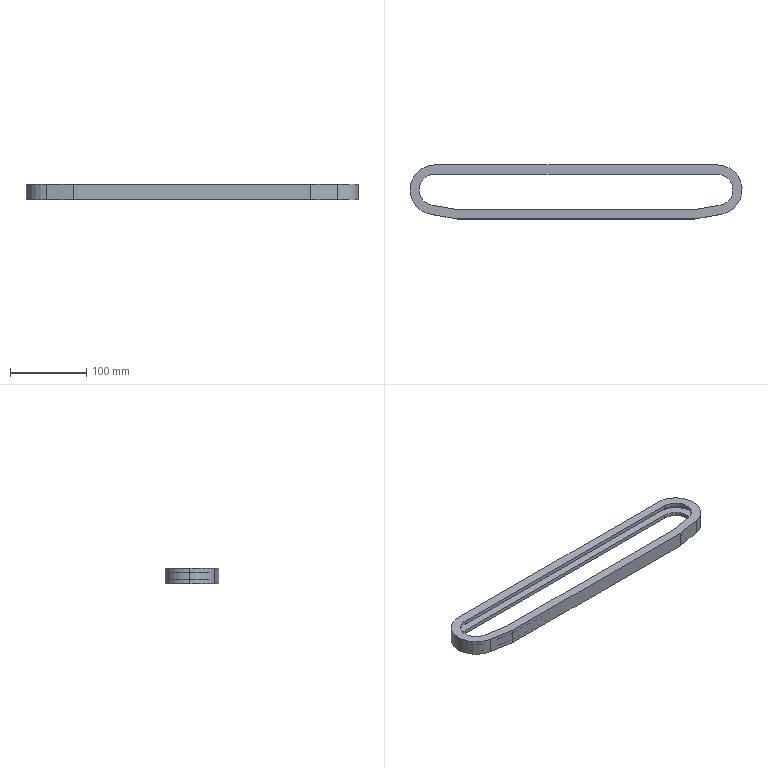Part | SolidWorks | features Extrusion 1, ICE 1 | 1 solid | 32 faces | box 435 x 70.699 x 20 mm | volume 118324 mm3 | plane 20 | cylinder 12 | commonest cylinder face diameters 41 x6 63 x3 65 x3
STEP:
#1=CARTESIAN_POINT('',(216.5,0.,-5.));
#2=VERTEX_POINT('',#1);
#3=CARTESIAN_POINT('',(185.,31.5,-5.));
#4=VERTEX_POINT('',#3);
#5=CARTESIAN_POINT('',(185.,0.,-5.));
#6=DIRECTION('',(0.,0.,1.));
#7=DIRECTION('',(1.,0.,0.));
#8=AXIS2_PLACEMENT_3D('',#5,#6,#7);
#9=CIRCLE('',#8,31.5);
#10=EDGE_CURVE('',#2,#4,#9,.T.);
#11=ORIENTED_EDGE('',*,*,#10,.F.);
#12=CARTESIAN_POINT('',(216.5,0.,5.));
#13=VERTEX_POINT('',#12);
#14=CARTESIAN_POINT('',(216.5,0.,-5.));
#15=DIRECTION('',(0.,0.,1.));
#16=VECTOR('',#15,1000.);
#17=LINE('',#14,#16);
#18=EDGE_CURVE('',#2,#13,#17,.T.);
#19=ORIENTED_EDGE('',*,*,#18,.T.);
#20=CARTESIAN_POINT('',(185.,31.5,5.));
#21=VERTEX_POINT('',#20);
#22=CARTESIAN_POINT('',(185.,0.,5.));
#23=DIRECTION('',(0.,0.,1.));
#24=DIRECTION('',(1.,0.,0.));
#25=AXIS2_PLACEMENT_3D('',#22,#23,#24);
#26=CIRCLE('',#25,31.5);
#27=EDGE_CURVE('',#13,#21,#26,.T.);
#28=ORIENTED_EDGE('',*,*,#27,.T.);
#29=CARTESIAN_POINT('',(185.,31.5,-5.));
#30=DIRECTION('',(0.,0.,1.));
#31=VECTOR('',#30,1000.);
#32=LINE('',#29,#31);
#33=EDGE_CURVE('',#4,#21,#32,.T.);
#34=ORIENTED_EDGE('',*,*,#33,.F.);
#35=EDGE_LOOP('',(#11,#19,#28,#34));
#36=FACE_OUTER_BOUND('',#35,.T.);
#37=CARTESIAN_POINT('',(185.,0.,-5.));
#38=DIRECTION('',(0.,0.,1.));
#39=DIRECTION('',(1.,0.,0.));
#40=AXIS2_PLACEMENT_3D('',#37,#38,#39);
#41=CYLINDRICAL_SURFACE('',#40,31.5);
#42=ADVANCED_FACE('',(#36),#41,.F.);
#43=CARTESIAN_POINT('',(-185.,20.5,10.));
#44=VERTEX_POINT('',#43);
#45=CARTESIAN_POINT('',(-205.5,0.,10.));
#46=VERTEX_POINT('',#45);
#47=CARTESIAN_POINT('',(-185.,0.,10.));
#48=DIRECTION('',(0.,0.,1.));
#49=DIRECTION('',(1.,0.,0.));
#50=AXIS2_PLACEMENT_3D('',#47,#48,#49);
#51=CIRCLE('',#50,20.5);
#52=EDGE_CURVE('',#44,#46,#51,.T.);
#53=ORIENTED_EDGE('',*,*,#52,.T.);
#54=CARTESIAN_POINT('',(-205.5,0.,5.));
#55=VERTEX_POINT('',#54);
#56=CARTESIAN_POINT('',(-205.5,0.,10.));
#57=DIRECTION('',(0.,0.,-1.));
#58=VECTOR('',#57,1000.);
#59=LINE('',#56,#58);
#60=EDGE_CURVE('',#46,#55,#59,.T.);
#61=ORIENTED_EDGE('',*,*,#60,.T.);
#62=CARTESIAN_POINT('',(-185.,20.5,5.));
#63=VERTEX_POINT('',#62);
#64=CARTESIAN_POINT('',(-185.,0.,5.));
#65=DIRECTION('',(0.,0.,1.));
#66=DIRECTION('',(1.,0.,0.));
#67=AXIS2_PLACEMENT_3D('',#64,#65,#66);
#68=CIRCLE('',#67,20.5);
#69=EDGE_CURVE('',#63,#55,#68,.T.);
#70=ORIENTED_EDGE('',*,*,#69,.F.);
#71=CARTESIAN_POINT('',(-185.,20.5,10.));
#72=DIRECTION('',(0.,0.,-1.));
#73=VECTOR('',#72,1000.);
#74=LINE('',#71,#73);
#75=EDGE_CURVE('',#44,#63,#74,.T.);
#76=ORIENTED_EDGE('',*,*,#75,.F.);
#77=EDGE_LOOP('',(#53,#61,#70,#76));
#78=FACE_OUTER_BOUND('',#77,.T.);
#79=CARTESIAN_POINT('',(-185.,0.,10.));
#80=DIRECTION('',(0.,0.,-1.));
#81=DIRECTION('',(-1.,0.,0.));
#82=AXIS2_PLACEMENT_3D('',#79,#80,#81);
#83=CYLINDRICAL_SURFACE('',#82,20.5);
#84=ADVANCED_FACE('',(#78),#83,.F.);
#85=CARTESIAN_POINT('',(-217.5,0.,10.));
#86=VERTEX_POINT('',#85);
#87=CARTESIAN_POINT('',(-190.644,-32.006,10.));
#88=VERTEX_POINT('',#87);
#89=CARTESIAN_POINT('',(-185.,0.,10.));
#90=DIRECTION('',(0.,0.,1.));
#91=DIRECTION('',(1.,0.,0.));
#92=AXIS2_PLACEMENT_3D('',#89,#90,#91);
#93=CIRCLE('',#92,32.5);
#94=EDGE_CURVE('',#86,#88,#93,.T.);
#95=ORIENTED_EDGE('',*,*,#94,.F.);
#96=CARTESIAN_POINT('',(-217.5,0.,-10.));
#97=VERTEX_POINT('',#96);
#98=CARTESIAN_POINT('',(-217.5,0.,10.));
#99=DIRECTION('',(0.,0.,-1.));
#100=VECTOR('',#99,1000.);
#101=LINE('',#98,#100);
#102=EDGE_CURVE('',#86,#97,#101,.T.);
#103=ORIENTED_EDGE('',*,*,#102,.T.);
#104=CARTESIAN_POINT('',(-190.644,-32.006,-10.));
#105=VERTEX_POINT('',#104);
#106=CARTESIAN_POINT('',(-185.,0.,-10.));
#107=DIRECTION('',(0.,0.,1.));
#108=DIRECTION('',(1.,0.,0.));
#109=AXIS2_PLACEMENT_3D('',#106,#107,#108);
#110=CIRCLE('',#109,32.5);
#111=EDGE_CURVE('',#97,#105,#110,.T.);
#112=ORIENTED_EDGE('',*,*,#111,.T.);
#113=CARTESIAN_POINT('',(-190.644,-32.006,10.));
#114=DIRECTION('',(0.,0.,-1.));
#115=VECTOR('',#114,1000.);
#116=LINE('',#113,#115);
#117=EDGE_CURVE('',#88,#105,#116,.T.);
#118=ORIENTED_EDGE('',*,*,#117,.F.);
#119=EDGE_LOOP('',(#95,#103,#112,#118));
#120=FACE_OUTER_BOUND('',#119,.T.);
#121=CARTESIAN_POINT('',(-185.,0.,10.));
#122=DIRECTION('',(0.,0.,-1.));
#123=DIRECTION('',(-1.,0.,0.));
#124=AXIS2_PLACEMENT_3D('',#121,#122,#123);
#125=CYLINDRICAL_SURFACE('',#124,32.5);
#126=ADVANCED_FACE('',(#120),#125,.T.);
#127=CARTESIAN_POINT('',(-185.,20.5,-5.));
#128=VERTEX_POINT('',#127);
#129=CARTESIAN_POINT('',(-205.5,0.,-5.));
#130=VERTEX_POINT('',#129);
#131=CARTESIAN_POINT('',(-185.,0.,-5.));
#132=DIRECTION('',(0.,0.,1.));
#133=DIRECTION('',(1.,0.,0.));
#134=AXIS2_PLACEMENT_3D('',#131,#132,#133);
#135=CIRCLE('',#134,20.5);
#136=EDGE_CURVE('',#128,#130,#135,.T.);
#137=ORIENTED_EDGE('',*,*,#136,.T.);
#138=CARTESIAN_POINT('',(-205.5,0.,-10.));
#139=VERTEX_POINT('',#138);
#140=CARTESIAN_POINT('',(-205.5,0.,10.));
#141=DIRECTION('',(0.,0.,-1.));
#142=VECTOR('',#141,1000.);
#143=LINE('',#140,#142);
#144=EDGE_CURVE('',#130,#139,#143,.T.);
#145=ORIENTED_EDGE('',*,*,#144,.T.);
#146=CARTESIAN_POINT('',(-185.,20.5,-10.));
#147=VERTEX_POINT('',#146);
#148=CARTESIAN_POINT('',(-185.,0.,-10.));
#149=DIRECTION('',(0.,0.,1.));
#150=DIRECTION('',(1.,0.,0.));
#151=AXIS2_PLACEMENT_3D('',#148,#149,#150);
#152=CIRCLE('',#151,20.5);
#153=EDGE_CURVE('',#147,#139,#152,.T.);
#154=ORIENTED_EDGE('',*,*,#153,.F.);
#155=CARTESIAN_POINT('',(-185.,20.5,10.));
#156=DIRECTION('',(0.,0.,-1.));
#157=VECTOR('',#156,1000.);
#158=LINE('',#155,#157);
#159=EDGE_CURVE('',#128,#147,#158,.T.);
#160=ORIENTED_EDGE('',*,*,#159,.F.);
#161=EDGE_LOOP('',(#137,#145,#154,#160));
#162=FACE_OUTER_BOUND('',#161,.T.);
#163=CARTESIAN_POINT('',(-185.,0.,10.));
#164=DIRECTION('',(0.,0.,-1.));
#165=DIRECTION('',(-1.,0.,0.));
#166=AXIS2_PLACEMENT_3D('',#163,#164,#165);
#167=CYLINDRICAL_SURFACE('',#166,20.5);
#168=ADVANCED_FACE('',(#162),#167,.F.);
#169=ORIENTED_EDGE('',*,*,#144,.F.);
#170=CARTESIAN_POINT('',(-188.56,-20.189,-5.));
#171=VERTEX_POINT('',#170);
#172=CARTESIAN_POINT('',(-185.,0.,-5.));
#173=DIRECTION('',(0.,0.,1.));
#174=DIRECTION('',(1.,0.,0.));
#175=AXIS2_PLACEMENT_3D('',#172,#173,#174);
#176=CIRCLE('',#175,20.5);
#177=EDGE_CURVE('',#130,#171,#176,.T.);
#178=ORIENTED_EDGE('',*,*,#177,.T.);
#179=CARTESIAN_POINT('',(-188.56,-20.189,-10.));
#180=VERTEX_POINT('',#179);
#181=CARTESIAN_POINT('',(-188.56,-20.189,10.));
#182=DIRECTION('',(0.,0.,-1.));
#183=VECTOR('',#182,1000.);
#184=LINE('',#181,#183);
#185=EDGE_CURVE('',#171,#180,#184,.T.);
#186=ORIENTED_EDGE('',*,*,#185,.T.);
#187=CARTESIAN_POINT('',(-185.,0.,-10.));
#188=DIRECTION('',(0.,0.,1.));
#189=DIRECTION('',(1.,0.,0.));
#190=AXIS2_PLACEMENT_3D('',#187,#188,#189);
#191=CIRCLE('',#190,20.5);
#192=EDGE_CURVE('',#139,#180,#191,.T.);
#193=ORIENTED_EDGE('',*,*,#192,.F.);
#194=EDGE_LOOP('',(#169,#178,#186,#193));
#195=FACE_OUTER_BOUND('',#194,.T.);
#196=CARTESIAN_POINT('',(-185.,0.,10.));
#197=DIRECTION('',(0.,0.,-1.));
#198=DIRECTION('',(-1.,0.,0.));
#199=AXIS2_PLACEMENT_3D('',#196,#197,#198);
#200=CYLINDRICAL_SURFACE('',#199,20.5);
#201=ADVANCED_FACE('',(#195),#200,.F.);
#202=ORIENTED_EDGE('',*,*,#185,.F.);
#203=CARTESIAN_POINT('',(-154.475,-26.199,-5.));
#204=VERTEX_POINT('',#203);
#205=CARTESIAN_POINT('',(-154.475,-26.199,-5.));
#206=DIRECTION('',(0.9848,-0.1736,0.));
#207=VECTOR('',#206,1000.);
#208=LINE('',#205,#207);
#209=EDGE_CURVE('',#171,#204,#208,.T.);
#210=ORIENTED_EDGE('',*,*,#209,.T.);
#211=CARTESIAN_POINT('',(-154.475,-26.199,-10.));
#212=VERTEX_POINT('',#211);
#213=CARTESIAN_POINT('',(-154.475,-26.199,10.));
#214=DIRECTION('',(0.,0.,-1.));
#215=VECTOR('',#214,1000.);
#216=LINE('',#213,#215);
#217=EDGE_CURVE('',#204,#212,#216,.T.);
#218=ORIENTED_EDGE('',*,*,#217,.T.);
#219=CARTESIAN_POINT('',(-154.475,-26.199,-10.));
#220=DIRECTION('',(0.9848,-0.1736,0.));
#221=VECTOR('',#220,1000.);
#222=LINE('',#219,#221);
#223=EDGE_CURVE('',#180,#212,#222,.T.);
#224=ORIENTED_EDGE('',*,*,#223,.F.);
#225=EDGE_LOOP('',(#202,#210,#218,#224));
#226=FACE_OUTER_BOUND('',#225,.T.);
#227=CARTESIAN_POINT('',(-154.475,-26.199,10.));
#228=DIRECTION('',(0.1736,0.9848,0.));
#229=DIRECTION('',(-0.9848,0.1736,0.));
#230=AXIS2_PLACEMENT_3D('',#227,#228,#229);
#231=PLANE('',#230);
#232=ADVANCED_FACE('',(#226),#231,.T.);
#233=ORIENTED_EDGE('',*,*,#217,.F.);
#234=CARTESIAN_POINT('',(154.475,-26.199,-5.));
#235=VERTEX_POINT('',#234);
#236=CARTESIAN_POINT('',(-154.475,-26.199,-5.));
#237=DIRECTION('',(1.,0.,0.));
#238=VECTOR('',#237,1000.);
#239=LINE('',#236,#238);
#240=EDGE_CURVE('',#204,#235,#239,.T.);
#241=ORIENTED_EDGE('',*,*,#240,.T.);
#242=CARTESIAN_POINT('',(154.475,-26.199,-10.));
#243=VERTEX_POINT('',#242);
#244=CARTESIAN_POINT('',(154.475,-26.199,10.));
#245=DIRECTION('',(0.,0.,-1.));
#246=VECTOR('',#245,1000.);
#247=LINE('',#244,#246);
#248=EDGE_CURVE('',#235,#243,#247,.T.);
#249=ORIENTED_EDGE('',*,*,#248,.T.);
#250=CARTESIAN_POINT('',(-154.475,-26.199,-10.));
#251=DIRECTION('',(1.,0.,0.));
#252=VECTOR('',#251,1000.);
#253=LINE('',#250,#252);
#254=EDGE_CURVE('',#212,#243,#253,.T.);
#255=ORIENTED_EDGE('',*,*,#254,.F.);
#256=EDGE_LOOP('',(#233,#241,#249,#255));
#257=FACE_OUTER_BOUND('',#256,.T.);
#258=CARTESIAN_POINT('',(-154.475,-26.199,10.));
#259=DIRECTION('',(0.,1.,0.));
#260=DIRECTION('',(0.,0.,1.));
#261=AXIS2_PLACEMENT_3D('',#258,#259,#260);
#262=PLANE('',#261);
#263=ADVANCED_FACE('',(#257),#262,.T.);
#264=ORIENTED_EDGE('',*,*,#248,.F.);
#265=CARTESIAN_POINT('',(188.56,-20.189,-5.));
#266=VERTEX_POINT('',#265);
#267=CARTESIAN_POINT('',(154.475,-26.199,-5.));
#268=DIRECTION('',(0.9848,0.1736,0.));
#269=VECTOR('',#268,1000.);
#270=LINE('',#267,#269);
#271=EDGE_CURVE('',#235,#266,#270,.T.);
#272=ORIENTED_EDGE('',*,*,#271,.T.);
#273=CARTESIAN_POINT('',(188.56,-20.189,-10.));
#274=VERTEX_POINT('',#273);
#275=CARTESIAN_POINT('',(188.56,-20.189,10.));
#276=DIRECTION('',(0.,0.,-1.));
#277=VECTOR('',#276,1000.);
#278=LINE('',#275,#277);
#279=EDGE_CURVE('',#266,#274,#278,.T.);
#280=ORIENTED_EDGE('',*,*,#279,.T.);
#281=CARTESIAN_POINT('',(154.475,-26.199,-10.));
#282=DIRECTION('',(0.9848,0.1736,0.));
#283=VECTOR('',#282,1000.);
#284=LINE('',#281,#283);
#285=EDGE_CURVE('',#243,#274,#284,.T.);
#286=ORIENTED_EDGE('',*,*,#285,.F.);
#287=EDGE_LOOP('',(#264,#272,#280,#286));
#288=FACE_OUTER_BOUND('',#287,.T.);
#289=CARTESIAN_POINT('',(154.475,-26.199,10.));
#290=DIRECTION('',(-0.1736,0.9848,0.));
#291=DIRECTION('',(-0.9848,-0.1736,0.));
#292=AXIS2_PLACEMENT_3D('',#289,#290,#291);
#293=PLANE('',#292);
#294=ADVANCED_FACE('',(#288),#293,.T.);
#295=ORIENTED_EDGE('',*,*,#279,.F.);
#296=CARTESIAN_POINT('',(185.,20.5,-5.));
#297=VERTEX_POINT('',#296);
#298=CARTESIAN_POINT('',(185.,0.,-5.));
#299=DIRECTION('',(0.,0.,1.));
#300=DIRECTION('',(1.,0.,0.));
#301=AXIS2_PLACEMENT_3D('',#298,#299,#300);
#302=CIRCLE('',#301,20.5);
#303=EDGE_CURVE('',#266,#297,#302,.T.);
#304=ORIENTED_EDGE('',*,*,#303,.T.);
#305=CARTESIAN_POINT('',(185.,20.5,-10.));
#306=VERTEX_POINT('',#305);
#307=CARTESIAN_POINT('',(185.,20.5,10.));
#308=DIRECTION('',(0.,0.,-1.));
#309=VECTOR('',#308,1000.);
#310=LINE('',#307,#309);
#311=EDGE_CURVE('',#297,#306,#310,.T.);
#312=ORIENTED_EDGE('',*,*,#311,.T.);
#313=CARTESIAN_POINT('',(185.,0.,-10.));
#314=DIRECTION('',(0.,0.,1.));
#315=DIRECTION('',(-1.,0.,0.));
#316=AXIS2_PLACEMENT_3D('',#313,#314,#315);
#317=CIRCLE('',#316,20.5);
#318=EDGE_CURVE('',#274,#306,#317,.T.);
#319=ORIENTED_EDGE('',*,*,#318,.F.);
#320=EDGE_LOOP('',(#295,#304,#312,#319));
#321=FACE_OUTER_BOUND('',#320,.T.);
#322=CARTESIAN_POINT('',(185.,0.,10.));
#323=DIRECTION('',(0.,0.,-1.));
#324=DIRECTION('',(-1.,0.,0.));
#325=AXIS2_PLACEMENT_3D('',#322,#323,#324);
#326=CYLINDRICAL_SURFACE('',#325,20.5);
#327=ADVANCED_FACE('',(#321),#326,.F.);
#328=ORIENTED_EDGE('',*,*,#311,.F.);
#329=CARTESIAN_POINT('',(-185.,20.5,-5.));
#330=DIRECTION('',(-1.,0.,0.));
#331=VECTOR('',#330,1000.);
#332=LINE('',#329,#331);
#333=EDGE_CURVE('',#297,#128,#332,.T.);
#334=ORIENTED_EDGE('',*,*,#333,.T.);
#335=ORIENTED_EDGE('',*,*,#159,.T.);
#336=CARTESIAN_POINT('',(-185.,20.5,-10.));
#337=DIRECTION('',(-1.,0.,0.));
#338=VECTOR('',#337,1000.);
#339=LINE('',#336,#338);
#340=EDGE_CURVE('',#306,#147,#339,.T.);
#341=ORIENTED_EDGE('',*,*,#340,.F.);
#342=EDGE_LOOP('',(#328,#334,#335,#341));
#343=FACE_OUTER_BOUND('',#342,.T.);
#344=CARTESIAN_POINT('',(-185.,20.5,10.));
#345=DIRECTION('',(0.,-1.,0.));
#346=DIRECTION('',(0.,0.,-1.));
#347=AXIS2_PLACEMENT_3D('',#344,#345,#346);
#348=PLANE('',#347);
#349=ADVANCED_FACE('',(#343),#348,.T.);
#350=CARTESIAN_POINT('',(-185.,32.5,10.));
#351=VERTEX_POINT('',#350);
#352=CARTESIAN_POINT('',(-185.,0.,10.));
#353=DIRECTION('',(0.,0.,1.));
#354=DIRECTION('',(1.,0.,0.));
#355=AXIS2_PLACEMENT_3D('',#352,#353,#354);
#356=CIRCLE('',#355,32.5);
#357=EDGE_CURVE('',#351,#86,#356,.T.);
#358=ORIENTED_EDGE('',*,*,#357,.T.);
#359=ORIENTED_EDGE('',*,*,#94,.T.);
#360=CARTESIAN_POINT('',(-155.525,-38.199,10.));
#361=VERTEX_POINT('',#360);
#362=CARTESIAN_POINT('',(-155.525,-38.199,10.));
#363=DIRECTION('',(0.9848,-0.1736,0.));
#364=VECTOR('',#363,1000.);
#365=LINE('',#362,#364);
#366=EDGE_CURVE('',#88,#361,#365,.T.);
#367=ORIENTED_EDGE('',*,*,#366,.T.);
#368=CARTESIAN_POINT('',(155.525,-38.199,10.));
#369=VERTEX_POINT('',#368);
#370=CARTESIAN_POINT('',(-155.525,-38.199,10.));
#371=DIRECTION('',(1.,0.,0.));
#372=VECTOR('',#371,1000.);
#373=LINE('',#370,#372);
#374=EDGE_CURVE('',#361,#369,#373,.T.);
#375=ORIENTED_EDGE('',*,*,#374,.T.);
#376=CARTESIAN_POINT('',(190.644,-32.006,10.));
#377=VERTEX_POINT('',#376);
#378=CARTESIAN_POINT('',(155.525,-38.199,10.));
#379=DIRECTION('',(0.9848,0.1736,0.));
#380=VECTOR('',#379,1000.);
#381=LINE('',#378,#380);
#382=EDGE_CURVE('',#369,#377,#381,.T.);
#383=ORIENTED_EDGE('',*,*,#382,.T.);
#384=CARTESIAN_POINT('',(185.,32.5,10.));
#385=VERTEX_POINT('',#384);
#386=CARTESIAN_POINT('',(185.,0.,10.));
#387=DIRECTION('',(0.,0.,1.));
#388=DIRECTION('',(-1.,0.,0.));
#389=AXIS2_PLACEMENT_3D('',#386,#387,#388);
#390=CIRCLE('',#389,32.5);
#391=EDGE_CURVE('',#377,#385,#390,.T.);
#392=ORIENTED_EDGE('',*,*,#391,.T.);
#393=CARTESIAN_POINT('',(-185.,32.5,10.));
#394=DIRECTION('',(-1.,0.,0.));
#395=VECTOR('',#394,1000.);
#396=LINE('',#393,#395);
#397=EDGE_CURVE('',#385,#351,#396,.T.);
#398=ORIENTED_EDGE('',*,*,#397,.T.);
#399=EDGE_LOOP('',(#358,#359,#367,#375,#383,#392,#398));
#400=FACE_OUTER_BOUND('',#399,.T.);
#401=CARTESIAN_POINT('',(-188.56,-20.189,10.));
#402=VERTEX_POINT('',#401);
#403=CARTESIAN_POINT('',(-154.475,-26.199,10.));
#404=VERTEX_POINT('',#403);
#405=CARTESIAN_POINT('',(-154.475,-26.199,10.));
#406=DIRECTION('',(0.9848,-0.1736,0.));
#407=VECTOR('',#406,1000.);
#408=LINE('',#405,#407);
#409=EDGE_CURVE('',#402,#404,#408,.T.);
#410=ORIENTED_EDGE('',*,*,#409,.F.);
#411=CARTESIAN_POINT('',(-185.,0.,10.));
#412=DIRECTION('',(0.,0.,1.));
#413=DIRECTION('',(1.,0.,0.));
#414=AXIS2_PLACEMENT_3D('',#411,#412,#413);
#415=CIRCLE('',#414,20.5);
#416=EDGE_CURVE('',#46,#402,#415,.T.);
#417=ORIENTED_EDGE('',*,*,#416,.F.);
#418=ORIENTED_EDGE('',*,*,#52,.F.);
#419=CARTESIAN_POINT('',(185.,20.5,10.));
#420=VERTEX_POINT('',#419);
#421=CARTESIAN_POINT('',(-185.,20.5,10.));
#422=DIRECTION('',(-1.,0.,0.));
#423=VECTOR('',#422,1000.);
#424=LINE('',#421,#423);
#425=EDGE_CURVE('',#420,#44,#424,.T.);
#426=ORIENTED_EDGE('',*,*,#425,.F.);
#427=CARTESIAN_POINT('',(188.56,-20.189,10.));
#428=VERTEX_POINT('',#427);
#429=CARTESIAN_POINT('',(185.,0.,10.));
#430=DIRECTION('',(0.,0.,1.));
#431=DIRECTION('',(-1.,0.,0.));
#432=AXIS2_PLACEMENT_3D('',#429,#430,#431);
#433=CIRCLE('',#432,20.5);
#434=EDGE_CURVE('',#428,#420,#433,.T.);
#435=ORIENTED_EDGE('',*,*,#434,.F.);
#436=CARTESIAN_POINT('',(154.475,-26.199,10.));
#437=VERTEX_POINT('',#436);
#438=CARTESIAN_POINT('',(154.475,-26.199,10.));
#439=DIRECTION('',(0.9848,0.1736,0.));
#440=VECTOR('',#439,1000.);
#441=LINE('',#438,#440);
#442=EDGE_CURVE('',#437,#428,#441,.T.);
#443=ORIENTED_EDGE('',*,*,#442,.F.);
#444=CARTESIAN_POINT('',(-154.475,-26.199,10.));
#445=DIRECTION('',(1.,0.,0.));
#446=VECTOR('',#445,1000.);
#447=LINE('',#444,#446);
#448=EDGE_CURVE('',#404,#437,#447,.T.);
#449=ORIENTED_EDGE('',*,*,#448,.F.);
#450=EDGE_LOOP('',(#410,#417,#418,#426,#435,#443,#449));
#451=FACE_BOUND('',#450,.T.);
#452=CARTESIAN_POINT('',(-185.,0.,10.));
#453=DIRECTION('',(0.,0.,1.));
#454=DIRECTION('',(1.,0.,0.));
#455=AXIS2_PLACEMENT_3D('',#452,#453,#454);
#456=PLANE('',#455);
#457=ADVANCED_FACE('',(#400,#451),#456,.T.);
#458=CARTESIAN_POINT('',(-185.,32.5,-10.));
#459=VERTEX_POINT('',#458);
#460=CARTESIAN_POINT('',(-185.,0.,-10.));
#461=DIRECTION('',(0.,0.,1.));
#462=DIRECTION('',(1.,0.,0.));
#463=AXIS2_PLACEMENT_3D('',#460,#461,#462);
#464=CIRCLE('',#463,32.5);
#465=EDGE_CURVE('',#459,#97,#464,.T.);
#466=ORIENTED_EDGE('',*,*,#465,.F.);
#467=CARTESIAN_POINT('',(185.,32.5,-10.));
#468=VERTEX_POINT('',#467);
#469=CARTESIAN_POINT('',(-185.,32.5,-10.));
#470=DIRECTION('',(-1.,0.,0.));
#471=VECTOR('',#470,1000.);
#472=LINE('',#469,#471);
#473=EDGE_CURVE('',#468,#459,#472,.T.);
#474=ORIENTED_EDGE('',*,*,#473,.F.);
#475=CARTESIAN_POINT('',(190.644,-32.006,-10.));
#476=VERTEX_POINT('',#475);
#477=CARTESIAN_POINT('',(185.,0.,-10.));
#478=DIRECTION('',(0.,0.,1.));
#479=DIRECTION('',(-1.,0.,0.));
#480=AXIS2_PLACEMENT_3D('',#477,#478,#479);
#481=CIRCLE('',#480,32.5);
#482=EDGE_CURVE('',#476,#468,#481,.T.);
#483=ORIENTED_EDGE('',*,*,#482,.F.);
#484=CARTESIAN_POINT('',(155.525,-38.199,-10.));
#485=VERTEX_POINT('',#484);
#486=CARTESIAN_POINT('',(155.525,-38.199,-10.));
#487=DIRECTION('',(0.9848,0.1736,0.));
#488=VECTOR('',#487,1000.);
#489=LINE('',#486,#488);
#490=EDGE_CURVE('',#485,#476,#489,.T.);
#491=ORIENTED_EDGE('',*,*,#490,.F.);
#492=CARTESIAN_POINT('',(-155.525,-38.199,-10.));
#493=VERTEX_POINT('',#492);
#494=CARTESIAN_POINT('',(-155.525,-38.199,-10.));
#495=DIRECTION('',(1.,0.,0.));
#496=VECTOR('',#495,1000.);
#497=LINE('',#494,#496);
#498=EDGE_CURVE('',#493,#485,#497,.T.);
#499=ORIENTED_EDGE('',*,*,#498,.F.);
#500=CARTESIAN_POINT('',(-155.525,-38.199,-10.));
#501=DIRECTION('',(0.9848,-0.1736,0.));
#502=VECTOR('',#501,1000.);
#503=LINE('',#500,#502);
#504=EDGE_CURVE('',#105,#493,#503,.T.);
#505=ORIENTED_EDGE('',*,*,#504,.F.);
#506=ORIENTED_EDGE('',*,*,#111,.F.);
#507=EDGE_LOOP('',(#466,#474,#483,#491,#499,#505,#506));
#508=FACE_OUTER_BOUND('',#507,.T.);
#509=ORIENTED_EDGE('',*,*,#153,.T.);
#510=ORIENTED_EDGE('',*,*,#192,.T.);
#511=ORIENTED_EDGE('',*,*,#223,.T.);
#512=ORIENTED_EDGE('',*,*,#254,.T.);
#513=ORIENTED_EDGE('',*,*,#285,.T.);
#514=ORIENTED_EDGE('',*,*,#318,.T.);
#515=ORIENTED_EDGE('',*,*,#340,.T.);
#516=EDGE_LOOP('',(#509,#510,#511,#512,#513,#514,#515));
#517=FACE_BOUND('',#516,.T.);
#518=CARTESIAN_POINT('',(-185.,0.,-10.));
#519=DIRECTION('',(0.,0.,1.));
#520=DIRECTION('',(1.,0.,0.));
#521=AXIS2_PLACEMENT_3D('',#518,#519,#520);
#522=PLANE('',#521);
#523=ADVANCED_FACE('',(#508,#517),#522,.F.);
#524=ORIENTED_EDGE('',*,*,#102,.F.);
#525=ORIENTED_EDGE('',*,*,#357,.F.);
#526=CARTESIAN_POINT('',(-185.,32.5,10.));
#527=DIRECTION('',(0.,0.,-1.));
#528=VECTOR('',#527,1000.);
#529=LINE('',#526,#528);
#530=EDGE_CURVE('',#351,#459,#529,.T.);
#531=ORIENTED_EDGE('',*,*,#530,.T.);
#532=ORIENTED_EDGE('',*,*,#465,.T.);
#533=EDGE_LOOP('',(#524,#525,#531,#532));
#534=FACE_OUTER_BOUND('',#533,.T.);
#535=CARTESIAN_POINT('',(-185.,0.,10.));
#536=DIRECTION('',(0.,0.,-1.));
#537=DIRECTION('',(-1.,0.,0.));
#538=AXIS2_PLACEMENT_3D('',#535,#536,#537);
#539=CYLINDRICAL_SURFACE('',#538,32.5);
#540=ADVANCED_FACE('',(#534),#539,.T.);
#541=ORIENTED_EDGE('',*,*,#504,.T.);
#542=CARTESIAN_POINT('',(-155.525,-38.199,10.));
#543=DIRECTION('',(0.,0.,-1.));
#544=VECTOR('',#543,1000.);
#545=LINE('',#542,#544);
#546=EDGE_CURVE('',#361,#493,#545,.T.);
#547=ORIENTED_EDGE('',*,*,#546,.F.);
#548=ORIENTED_EDGE('',*,*,#366,.F.);
#549=ORIENTED_EDGE('',*,*,#117,.T.);
#550=EDGE_LOOP('',(#541,#547,#548,#549));
#551=FACE_OUTER_BOUND('',#550,.T.);
#552=CARTESIAN_POINT('',(-155.525,-38.199,10.));
#553=DIRECTION('',(0.1736,0.9848,0.));
#554=DIRECTION('',(-0.9848,0.1736,0.));
#555=AXIS2_PLACEMENT_3D('',#552,#553,#554);
#556=PLANE('',#555);
#557=ADVANCED_FACE('',(#551),#556,.F.);
#558=ORIENTED_EDGE('',*,*,#498,.T.);
#559=CARTESIAN_POINT('',(155.525,-38.199,10.));
#560=DIRECTION('',(0.,0.,-1.));
#561=VECTOR('',#560,1000.);
#562=LINE('',#559,#561);
#563=EDGE_CURVE('',#369,#485,#562,.T.);
#564=ORIENTED_EDGE('',*,*,#563,.F.);
#565=ORIENTED_EDGE('',*,*,#374,.F.);
#566=ORIENTED_EDGE('',*,*,#546,.T.);
#567=EDGE_LOOP('',(#558,#564,#565,#566));
#568=FACE_OUTER_BOUND('',#567,.T.);
#569=CARTESIAN_POINT('',(-155.525,-38.199,10.));
#570=DIRECTION('',(0.,1.,0.));
#571=DIRECTION('',(0.,0.,1.));
#572=AXIS2_PLACEMENT_3D('',#569,#570,#571);
#573=PLANE('',#572);
#574=ADVANCED_FACE('',(#568),#573,.F.);
#575=ORIENTED_EDGE('',*,*,#490,.T.);
#576=CARTESIAN_POINT('',(190.644,-32.006,10.));
#577=DIRECTION('',(0.,0.,-1.));
#578=VECTOR('',#577,1000.);
#579=LINE('',#576,#578);
#580=EDGE_CURVE('',#377,#476,#579,.T.);
#581=ORIENTED_EDGE('',*,*,#580,.F.);
#582=ORIENTED_EDGE('',*,*,#382,.F.);
#583=ORIENTED_EDGE('',*,*,#563,.T.);
#584=EDGE_LOOP('',(#575,#581,#582,#583));
#585=FACE_OUTER_BOUND('',#584,.T.);
#586=CARTESIAN_POINT('',(155.525,-38.199,10.));
#587=DIRECTION('',(-0.1736,0.9848,0.));
#588=DIRECTION('',(-0.9848,-0.1736,0.));
#589=AXIS2_PLACEMENT_3D('',#586,#587,#588);
#590=PLANE('',#589);
#591=ADVANCED_FACE('',(#585),#590,.F.);
#592=ORIENTED_EDGE('',*,*,#482,.T.);
#593=CARTESIAN_POINT('',(185.,32.5,10.));
#594=DIRECTION('',(0.,0.,-1.));
#595=VECTOR('',#594,1000.);
#596=LINE('',#593,#595);
#597=EDGE_CURVE('',#385,#468,#596,.T.);
#598=ORIENTED_EDGE('',*,*,#597,.F.);
#599=ORIENTED_EDGE('',*,*,#391,.F.);
#600=ORIENTED_EDGE('',*,*,#580,.T.);
#601=EDGE_LOOP('',(#592,#598,#599,#600));
#602=FACE_OUTER_BOUND('',#601,.T.);
#603=CARTESIAN_POINT('',(185.,0.,10.));
#604=DIRECTION('',(0.,0.,-1.));
#605=DIRECTION('',(-1.,0.,0.));
#606=AXIS2_PLACEMENT_3D('',#603,#604,#605);
#607=CYLINDRICAL_SURFACE('',#606,32.5);
#608=ADVANCED_FACE('',(#602),#607,.T.);
#609=ORIENTED_EDGE('',*,*,#473,.T.);
#610=ORIENTED_EDGE('',*,*,#530,.F.);
#611=ORIENTED_EDGE('',*,*,#397,.F.);
#612=ORIENTED_EDGE('',*,*,#597,.T.);
#613=EDGE_LOOP('',(#609,#610,#611,#612));
#614=FACE_OUTER_BOUND('',#613,.T.);
#615=CARTESIAN_POINT('',(-185.,32.5,10.));
#616=DIRECTION('',(0.,-1.,0.));
#617=DIRECTION('',(0.,0.,-1.));
#618=AXIS2_PLACEMENT_3D('',#615,#616,#617);
#619=PLANE('',#618);
#620=ADVANCED_FACE('',(#614),#619,.F.);
#621=ORIENTED_EDGE('',*,*,#60,.F.);
#622=ORIENTED_EDGE('',*,*,#416,.T.);
#623=CARTESIAN_POINT('',(-188.56,-20.189,5.));
#624=VERTEX_POINT('',#623);
#625=CARTESIAN_POINT('',(-188.56,-20.189,10.));
#626=DIRECTION('',(0.,0.,-1.));
#627=VECTOR('',#626,1000.);
#628=LINE('',#625,#627);
#629=EDGE_CURVE('',#402,#624,#628,.T.);
#630=ORIENTED_EDGE('',*,*,#629,.T.);
#631=CARTESIAN_POINT('',(-185.,0.,5.));
#632=DIRECTION('',(0.,0.,1.));
#633=DIRECTION('',(1.,0.,0.));
#634=AXIS2_PLACEMENT_3D('',#631,#632,#633);
#635=CIRCLE('',#634,20.5);
#636=EDGE_CURVE('',#55,#624,#635,.T.);
#637=ORIENTED_EDGE('',*,*,#636,.F.);
#638=EDGE_LOOP('',(#621,#622,#630,#637));
#639=FACE_OUTER_BOUND('',#638,.T.);
#640=CARTESIAN_POINT('',(-185.,0.,10.));
#641=DIRECTION('',(0.,0.,-1.));
#642=DIRECTION('',(-1.,0.,0.));
#643=AXIS2_PLACEMENT_3D('',#640,#641,#642);
#644=CYLINDRICAL_SURFACE('',#643,20.5);
#645=ADVANCED_FACE('',(#639),#644,.F.);
#646=CARTESIAN_POINT('',(-154.475,-26.199,5.));
#647=VERTEX_POINT('',#646);
#648=CARTESIAN_POINT('',(-154.475,-26.199,5.));
#649=DIRECTION('',(0.9848,-0.1736,0.));
#650=VECTOR('',#649,1000.);
#651=LINE('',#648,#650);
#652=EDGE_CURVE('',#624,#647,#651,.T.);
#653=ORIENTED_EDGE('',*,*,#652,.F.);
#654=ORIENTED_EDGE('',*,*,#629,.F.);
#655=ORIENTED_EDGE('',*,*,#409,.T.);
#656=CARTESIAN_POINT('',(-154.475,-26.199,10.));
#657=DIRECTION('',(0.,0.,-1.));
#658=VECTOR('',#657,1000.);
#659=LINE('',#656,#658);
#660=EDGE_CURVE('',#404,#647,#659,.T.);
#661=ORIENTED_EDGE('',*,*,#660,.T.);
#662=EDGE_LOOP('',(#653,#654,#655,#661));
#663=FACE_OUTER_BOUND('',#662,.T.);
#664=CARTESIAN_POINT('',(-154.475,-26.199,10.));
#665=DIRECTION('',(0.1736,0.9848,0.));
#666=DIRECTION('',(-0.9848,0.1736,0.));
#667=AXIS2_PLACEMENT_3D('',#664,#665,#666);
#668=PLANE('',#667);
#669=ADVANCED_FACE('',(#663),#668,.T.);
#670=CARTESIAN_POINT('',(154.475,-26.199,5.));
#671=VERTEX_POINT('',#670);
#672=CARTESIAN_POINT('',(-154.475,-26.199,5.));
#673=DIRECTION('',(1.,0.,0.));
#674=VECTOR('',#673,1000.);
#675=LINE('',#672,#674);
#676=EDGE_CURVE('',#647,#671,#675,.T.);
#677=ORIENTED_EDGE('',*,*,#676,.F.);
#678=ORIENTED_EDGE('',*,*,#660,.F.);
#679=ORIENTED_EDGE('',*,*,#448,.T.);
#680=CARTESIAN_POINT('',(154.475,-26.199,10.));
#681=DIRECTION('',(0.,0.,-1.));
#682=VECTOR('',#681,1000.);
#683=LINE('',#680,#682);
#684=EDGE_CURVE('',#437,#671,#683,.T.);
#685=ORIENTED_EDGE('',*,*,#684,.T.);
#686=EDGE_LOOP('',(#677,#678,#679,#685));
#687=FACE_OUTER_BOUND('',#686,.T.);
#688=CARTESIAN_POINT('',(-154.475,-26.199,10.));
#689=DIRECTION('',(0.,1.,0.));
#690=DIRECTION('',(0.,0.,1.));
#691=AXIS2_PLACEMENT_3D('',#688,#689,#690);
#692=PLANE('',#691);
#693=ADVANCED_FACE('',(#687),#692,.T.);
#694=CARTESIAN_POINT('',(188.56,-20.189,5.));
#695=VERTEX_POINT('',#694);
#696=CARTESIAN_POINT('',(154.475,-26.199,5.));
#697=DIRECTION('',(0.9848,0.1736,0.));
#698=VECTOR('',#697,1000.);
#699=LINE('',#696,#698);
#700=EDGE_CURVE('',#671,#695,#699,.T.);
#701=ORIENTED_EDGE('',*,*,#700,.F.);
#702=ORIENTED_EDGE('',*,*,#684,.F.);
#703=ORIENTED_EDGE('',*,*,#442,.T.);
#704=CARTESIAN_POINT('',(188.56,-20.189,10.));
#705=DIRECTION('',(0.,0.,-1.));
#706=VECTOR('',#705,1000.);
#707=LINE('',#704,#706);
#708=EDGE_CURVE('',#428,#695,#707,.T.);
#709=ORIENTED_EDGE('',*,*,#708,.T.);
#710=EDGE_LOOP('',(#701,#702,#703,#709));
#711=FACE_OUTER_BOUND('',#710,.T.);
#712=CARTESIAN_POINT('',(154.475,-26.199,10.));
#713=DIRECTION('',(-0.1736,0.9848,0.));
#714=DIRECTION('',(-0.9848,-0.1736,0.));
#715=AXIS2_PLACEMENT_3D('',#712,#713,#714);
#716=PLANE('',#715);
#717=ADVANCED_FACE('',(#711),#716,.T.);
#718=CARTESIAN_POINT('',(185.,20.5,5.));
#719=VERTEX_POINT('',#718);
#720=CARTESIAN_POINT('',(185.,0.,5.));
#721=DIRECTION('',(0.,0.,1.));
#722=DIRECTION('',(1.,0.,0.));
#723=AXIS2_PLACEMENT_3D('',#720,#721,#722);
#724=CIRCLE('',#723,20.5);
#725=EDGE_CURVE('',#695,#719,#724,.T.);
#726=ORIENTED_EDGE('',*,*,#725,.F.);
#727=ORIENTED_EDGE('',*,*,#708,.F.);
#728=ORIENTED_EDGE('',*,*,#434,.T.);
#729=CARTESIAN_POINT('',(185.,20.5,10.));
#730=DIRECTION('',(0.,0.,-1.));
#731=VECTOR('',#730,1000.);
#732=LINE('',#729,#731);
#733=EDGE_CURVE('',#420,#719,#732,.T.);
#734=ORIENTED_EDGE('',*,*,#733,.T.);
#735=EDGE_LOOP('',(#726,#727,#728,#734));
#736=FACE_OUTER_BOUND('',#735,.T.);
#737=CARTESIAN_POINT('',(185.,0.,10.));
#738=DIRECTION('',(0.,0.,-1.));
#739=DIRECTION('',(-1.,0.,0.));
#740=AXIS2_PLACEMENT_3D('',#737,#738,#739);
#741=CYLINDRICAL_SURFACE('',#740,20.5);
#742=ADVANCED_FACE('',(#736),#741,.F.);
#743=CARTESIAN_POINT('',(-185.,20.5,5.));
#744=DIRECTION('',(-1.,0.,0.));
#745=VECTOR('',#744,1000.);
#746=LINE('',#743,#745);
#747=EDGE_CURVE('',#719,#63,#746,.T.);
#748=ORIENTED_EDGE('',*,*,#747,.F.);
#749=ORIENTED_EDGE('',*,*,#733,.F.);
#750=ORIENTED_EDGE('',*,*,#425,.T.);
#751=ORIENTED_EDGE('',*,*,#75,.T.);
#752=EDGE_LOOP('',(#748,#749,#750,#751));
#753=FACE_OUTER_BOUND('',#752,.T.);
#754=CARTESIAN_POINT('',(-185.,20.5,10.));
#755=DIRECTION('',(0.,-1.,0.));
#756=DIRECTION('',(0.,0.,-1.));
#757=AXIS2_PLACEMENT_3D('',#754,#755,#756);
#758=PLANE('',#757);
#759=ADVANCED_FACE('',(#753),#758,.T.);
#760=CARTESIAN_POINT('',(-155.437,-37.199,5.));
#761=VERTEX_POINT('',#760);
#762=CARTESIAN_POINT('',(155.437,-37.199,5.));
#763=VERTEX_POINT('',#762);
#764=CARTESIAN_POINT('',(-155.437,-37.199,5.));
#765=DIRECTION('',(1.,0.,0.));
#766=VECTOR('',#765,1000.);
#767=LINE('',#764,#766);
#768=EDGE_CURVE('',#761,#763,#767,.T.);
#769=ORIENTED_EDGE('',*,*,#768,.T.);
#770=CARTESIAN_POINT('',(155.437,-37.199,-5.));
#771=VERTEX_POINT('',#770);
#772=CARTESIAN_POINT('',(155.437,-37.199,-5.));
#773=DIRECTION('',(0.,0.,1.));
#774=VECTOR('',#773,1000.);
#775=LINE('',#772,#774);
#776=EDGE_CURVE('',#771,#763,#775,.T.);
#777=ORIENTED_EDGE('',*,*,#776,.F.);
#778=CARTESIAN_POINT('',(-155.437,-37.199,-5.));
#779=VERTEX_POINT('',#778);
#780=CARTESIAN_POINT('',(-155.437,-37.199,-5.));
#781=DIRECTION('',(1.,0.,0.));
#782=VECTOR('',#781,1000.);
#783=LINE('',#780,#782);
#784=EDGE_CURVE('',#779,#771,#783,.T.);
#785=ORIENTED_EDGE('',*,*,#784,.F.);
#786=CARTESIAN_POINT('',(-155.437,-37.199,-5.));
#787=DIRECTION('',(0.,0.,1.));
#788=VECTOR('',#787,1000.);
#789=LINE('',#786,#788);
#790=EDGE_CURVE('',#779,#761,#789,.T.);
#791=ORIENTED_EDGE('',*,*,#790,.T.);
#792=EDGE_LOOP('',(#769,#777,#785,#791));
#793=FACE_OUTER_BOUND('',#792,.T.);
#794=CARTESIAN_POINT('',(-155.437,-37.199,-5.));
#795=DIRECTION('',(0.,-1.,0.));
#796=DIRECTION('',(0.,0.,-1.));
#797=AXIS2_PLACEMENT_3D('',#794,#795,#796);
#798=PLANE('',#797);
#799=ADVANCED_FACE('',(#793),#798,.F.);
#800=CARTESIAN_POINT('',(-190.47,-31.021,5.));
#801=VERTEX_POINT('',#800);
#802=CARTESIAN_POINT('',(-190.47,-31.021,5.));
#803=DIRECTION('',(0.9848,-0.1736,0.));
#804=VECTOR('',#803,1000.);
#805=LINE('',#802,#804);
#806=EDGE_CURVE('',#801,#761,#805,.T.);
#807=ORIENTED_EDGE('',*,*,#806,.T.);
#808=ORIENTED_EDGE('',*,*,#790,.F.);
#809=CARTESIAN_POINT('',(-190.47,-31.021,-5.));
#810=VERTEX_POINT('',#809);
#811=CARTESIAN_POINT('',(-190.47,-31.021,-5.));
#812=DIRECTION('',(0.9848,-0.1736,0.));
#813=VECTOR('',#812,1000.);
#814=LINE('',#811,#813);
#815=EDGE_CURVE('',#810,#779,#814,.T.);
#816=ORIENTED_EDGE('',*,*,#815,.F.);
#817=CARTESIAN_POINT('',(-190.47,-31.021,-5.));
#818=DIRECTION('',(0.,0.,1.));
#819=VECTOR('',#818,1000.);
#820=LINE('',#817,#819);
#821=EDGE_CURVE('',#810,#801,#820,.T.);
#822=ORIENTED_EDGE('',*,*,#821,.T.);
#823=EDGE_LOOP('',(#807,#808,#816,#822));
#824=FACE_OUTER_BOUND('',#823,.T.);
#825=CARTESIAN_POINT('',(-190.47,-31.021,-5.));
#826=DIRECTION('',(-0.1736,-0.9848,0.));
#827=DIRECTION('',(0.9848,-0.1736,0.));
#828=AXIS2_PLACEMENT_3D('',#825,#826,#827);
#829=PLANE('',#828);
#830=ADVANCED_FACE('',(#824),#829,.F.);
#831=CARTESIAN_POINT('',(-185.,31.5,5.));
#832=VERTEX_POINT('',#831);
#833=CARTESIAN_POINT('',(-185.,0.,5.));
#834=DIRECTION('',(0.,0.,1.));
#835=DIRECTION('',(1.,0.,0.));
#836=AXIS2_PLACEMENT_3D('',#833,#834,#835);
#837=CIRCLE('',#836,31.5);
#838=EDGE_CURVE('',#832,#801,#837,.T.);
#839=ORIENTED_EDGE('',*,*,#838,.T.);
#840=ORIENTED_EDGE('',*,*,#821,.F.);
#841=CARTESIAN_POINT('',(-185.,31.5,-5.));
#842=VERTEX_POINT('',#841);
#843=CARTESIAN_POINT('',(-185.,0.,-5.));
#844=DIRECTION('',(0.,0.,1.));
#845=DIRECTION('',(1.,0.,0.));
#846=AXIS2_PLACEMENT_3D('',#843,#844,#845);
#847=CIRCLE('',#846,31.5);
#848=EDGE_CURVE('',#842,#810,#847,.T.);
#849=ORIENTED_EDGE('',*,*,#848,.F.);
#850=CARTESIAN_POINT('',(-185.,31.5,-5.));
#851=DIRECTION('',(0.,0.,1.));
#852=VECTOR('',#851,1000.);
#853=LINE('',#850,#852);
#854=EDGE_CURVE('',#842,#832,#853,.T.);
#855=ORIENTED_EDGE('',*,*,#854,.T.);
#856=EDGE_LOOP('',(#839,#840,#849,#855));
#857=FACE_OUTER_BOUND('',#856,.T.);
#858=CARTESIAN_POINT('',(-185.,0.,-5.));
#859=DIRECTION('',(0.,0.,1.));
#860=DIRECTION('',(1.,0.,0.));
#861=AXIS2_PLACEMENT_3D('',#858,#859,#860);
#862=CYLINDRICAL_SURFACE('',#861,31.5);
#863=ADVANCED_FACE('',(#857),#862,.F.);
#864=CARTESIAN_POINT('',(185.,31.5,5.));
#865=DIRECTION('',(-1.,0.,0.));
#866=VECTOR('',#865,1000.);
#867=LINE('',#864,#866);
#868=EDGE_CURVE('',#21,#832,#867,.T.);
#869=ORIENTED_EDGE('',*,*,#868,.T.);
#870=ORIENTED_EDGE('',*,*,#854,.F.);
#871=CARTESIAN_POINT('',(185.,31.5,-5.));
#872=DIRECTION('',(-1.,0.,0.));
#873=VECTOR('',#872,1000.);
#874=LINE('',#871,#873);
#875=EDGE_CURVE('',#4,#842,#874,.T.);
#876=ORIENTED_EDGE('',*,*,#875,.F.);
#877=ORIENTED_EDGE('',*,*,#33,.T.);
#878=EDGE_LOOP('',(#869,#870,#876,#877));
#879=FACE_OUTER_BOUND('',#878,.T.);
#880=CARTESIAN_POINT('',(185.,31.5,-5.));
#881=DIRECTION('',(0.,1.,0.));
#882=DIRECTION('',(-1.,0.,0.));
#883=AXIS2_PLACEMENT_3D('',#880,#881,#882);
#884=PLANE('',#883);
#885=ADVANCED_FACE('',(#879),#884,.F.);
#886=ORIENTED_EDGE('',*,*,#18,.F.);
#887=CARTESIAN_POINT('',(190.47,-31.021,-5.));
#888=VERTEX_POINT('',#887);
#889=CARTESIAN_POINT('',(185.,0.,-5.));
#890=DIRECTION('',(0.,0.,1.));
#891=DIRECTION('',(1.,0.,0.));
#892=AXIS2_PLACEMENT_3D('',#889,#890,#891);
#893=CIRCLE('',#892,31.5);
#894=EDGE_CURVE('',#888,#2,#893,.T.);
#895=ORIENTED_EDGE('',*,*,#894,.F.);
#896=CARTESIAN_POINT('',(190.47,-31.021,5.));
#897=VERTEX_POINT('',#896);
#898=CARTESIAN_POINT('',(190.47,-31.021,-5.));
#899=DIRECTION('',(0.,0.,1.));
#900=VECTOR('',#899,1000.);
#901=LINE('',#898,#900);
#902=EDGE_CURVE('',#888,#897,#901,.T.);
#903=ORIENTED_EDGE('',*,*,#902,.T.);
#904=CARTESIAN_POINT('',(185.,0.,5.));
#905=DIRECTION('',(0.,0.,1.));
#906=DIRECTION('',(1.,0.,0.));
#907=AXIS2_PLACEMENT_3D('',#904,#905,#906);
#908=CIRCLE('',#907,31.5);
#909=EDGE_CURVE('',#897,#13,#908,.T.);
#910=ORIENTED_EDGE('',*,*,#909,.T.);
#911=EDGE_LOOP('',(#886,#895,#903,#910));
#912=FACE_OUTER_BOUND('',#911,.T.);
#913=CARTESIAN_POINT('',(185.,0.,-5.));
#914=DIRECTION('',(0.,0.,1.));
#915=DIRECTION('',(1.,0.,0.));
#916=AXIS2_PLACEMENT_3D('',#913,#914,#915);
#917=CYLINDRICAL_SURFACE('',#916,31.5);
#918=ADVANCED_FACE('',(#912),#917,.F.);
#919=CARTESIAN_POINT('',(155.437,-37.199,5.));
#920=DIRECTION('',(0.9848,0.1736,0.));
#921=VECTOR('',#920,1000.);
#922=LINE('',#919,#921);
#923=EDGE_CURVE('',#763,#897,#922,.T.);
#924=ORIENTED_EDGE('',*,*,#923,.T.);
#925=ORIENTED_EDGE('',*,*,#902,.F.);
#926=CARTESIAN_POINT('',(155.437,-37.199,-5.));
#927=DIRECTION('',(0.9848,0.1736,0.));
#928=VECTOR('',#927,1000.);
#929=LINE('',#926,#928);
#930=EDGE_CURVE('',#771,#888,#929,.T.);
#931=ORIENTED_EDGE('',*,*,#930,.F.);
#932=ORIENTED_EDGE('',*,*,#776,.T.);
#933=EDGE_LOOP('',(#924,#925,#931,#932));
#934=FACE_OUTER_BOUND('',#933,.T.);
#935=CARTESIAN_POINT('',(155.437,-37.199,-5.));
#936=DIRECTION('',(0.1736,-0.9848,0.));
#937=DIRECTION('',(0.9848,0.1736,0.));
#938=AXIS2_PLACEMENT_3D('',#935,#936,#937);
#939=PLANE('',#938);
#940=ADVANCED_FACE('',(#934),#939,.F.);
#941=ORIENTED_EDGE('',*,*,#333,.F.);
#942=ORIENTED_EDGE('',*,*,#303,.F.);
#943=ORIENTED_EDGE('',*,*,#271,.F.);
#944=ORIENTED_EDGE('',*,*,#240,.F.);
#945=ORIENTED_EDGE('',*,*,#209,.F.);
#946=ORIENTED_EDGE('',*,*,#177,.F.);
#947=ORIENTED_EDGE('',*,*,#136,.F.);
#948=EDGE_LOOP('',(#941,#942,#943,#944,#945,#946,#947));
#949=FACE_BOUND('',#948,.T.);
#950=ORIENTED_EDGE('',*,*,#784,.T.);
#951=ORIENTED_EDGE('',*,*,#930,.T.);
#952=ORIENTED_EDGE('',*,*,#894,.T.);
#953=ORIENTED_EDGE('',*,*,#10,.T.);
#954=ORIENTED_EDGE('',*,*,#875,.T.);
#955=ORIENTED_EDGE('',*,*,#848,.T.);
#956=ORIENTED_EDGE('',*,*,#815,.T.);
#957=EDGE_LOOP('',(#950,#951,#952,#953,#954,#955,#956));
#958=FACE_OUTER_BOUND('',#957,.T.);
#959=CARTESIAN_POINT('',(185.,0.,-5.));
#960=DIRECTION('',(0.,0.,1.));
#961=DIRECTION('',(1.,0.,0.));
#962=AXIS2_PLACEMENT_3D('',#959,#960,#961);
#963=PLANE('',#962);
#964=ADVANCED_FACE('',(#949,#958),#963,.T.);
#965=ORIENTED_EDGE('',*,*,#69,.T.);
#966=ORIENTED_EDGE('',*,*,#636,.T.);
#967=ORIENTED_EDGE('',*,*,#652,.T.);
#968=ORIENTED_EDGE('',*,*,#676,.T.);
#969=ORIENTED_EDGE('',*,*,#700,.T.);
#970=ORIENTED_EDGE('',*,*,#725,.T.);
#971=ORIENTED_EDGE('',*,*,#747,.T.);
#972=EDGE_LOOP('',(#965,#966,#967,#968,#969,#970,#971));
#973=FACE_BOUND('',#972,.T.);
#974=ORIENTED_EDGE('',*,*,#768,.F.);
#975=ORIENTED_EDGE('',*,*,#806,.F.);
#976=ORIENTED_EDGE('',*,*,#838,.F.);
#977=ORIENTED_EDGE('',*,*,#868,.F.);
#978=ORIENTED_EDGE('',*,*,#27,.F.);
#979=ORIENTED_EDGE('',*,*,#909,.F.);
#980=ORIENTED_EDGE('',*,*,#923,.F.);
#981=EDGE_LOOP('',(#974,#975,#976,#977,#978,#979,#980));
#982=FACE_OUTER_BOUND('',#981,.T.);
#983=CARTESIAN_POINT('',(185.,0.,5.));
#984=DIRECTION('',(0.,0.,1.));
#985=DIRECTION('',(1.,0.,0.));
#986=AXIS2_PLACEMENT_3D('',#983,#984,#985);
#987=PLANE('',#986);
#988=ADVANCED_FACE('',(#973,#982),#987,.F.);
#989=CLOSED_SHELL('',(#42,#84,#126,#168,#201,#232,#263,#294,#327,#349,#457,#523,#540,#557,#574,#591,#608,#620,#645,#669,#693,#717,#742,#759,#799,#830,#863,#885,#918,#940,#964,#988));
#990=MANIFOLD_SOLID_BREP('',#989);
#991=CARTESIAN_POINT('',(0.,0.,0.));
#992=DIRECTION('',(0.,0.,1.));
#993=DIRECTION('',(1.,0.,0.));
#994=AXIS2_PLACEMENT_3D('',#991,#992,#993);
#995=(LENGTH_UNIT()NAMED_UNIT(*)SI_UNIT(.MILLI.,.METRE.));
#996=UNCERTAINTY_MEASURE_WITH_UNIT(LENGTH_MEASURE(0.00001),#995,'','');
#997=(NAMED_UNIT(*)PLANE_ANGLE_UNIT()SI_UNIT($,.RADIAN.));
#998=(NAMED_UNIT(*)SI_UNIT($,.STERADIAN.)SOLID_ANGLE_UNIT());
#999=(GEOMETRIC_REPRESENTATION_CONTEXT(3)GLOBAL_UNCERTAINTY_ASSIGNED_CONTEXT((#996))GLOBAL_UNIT_ASSIGNED_CONTEXT((#995,#997,#998))REPRESENTATION_CONTEXT('',''));
#1000=ADVANCED_BREP_SHAPE_REPRESENTATION('',(#990,#994),#999);